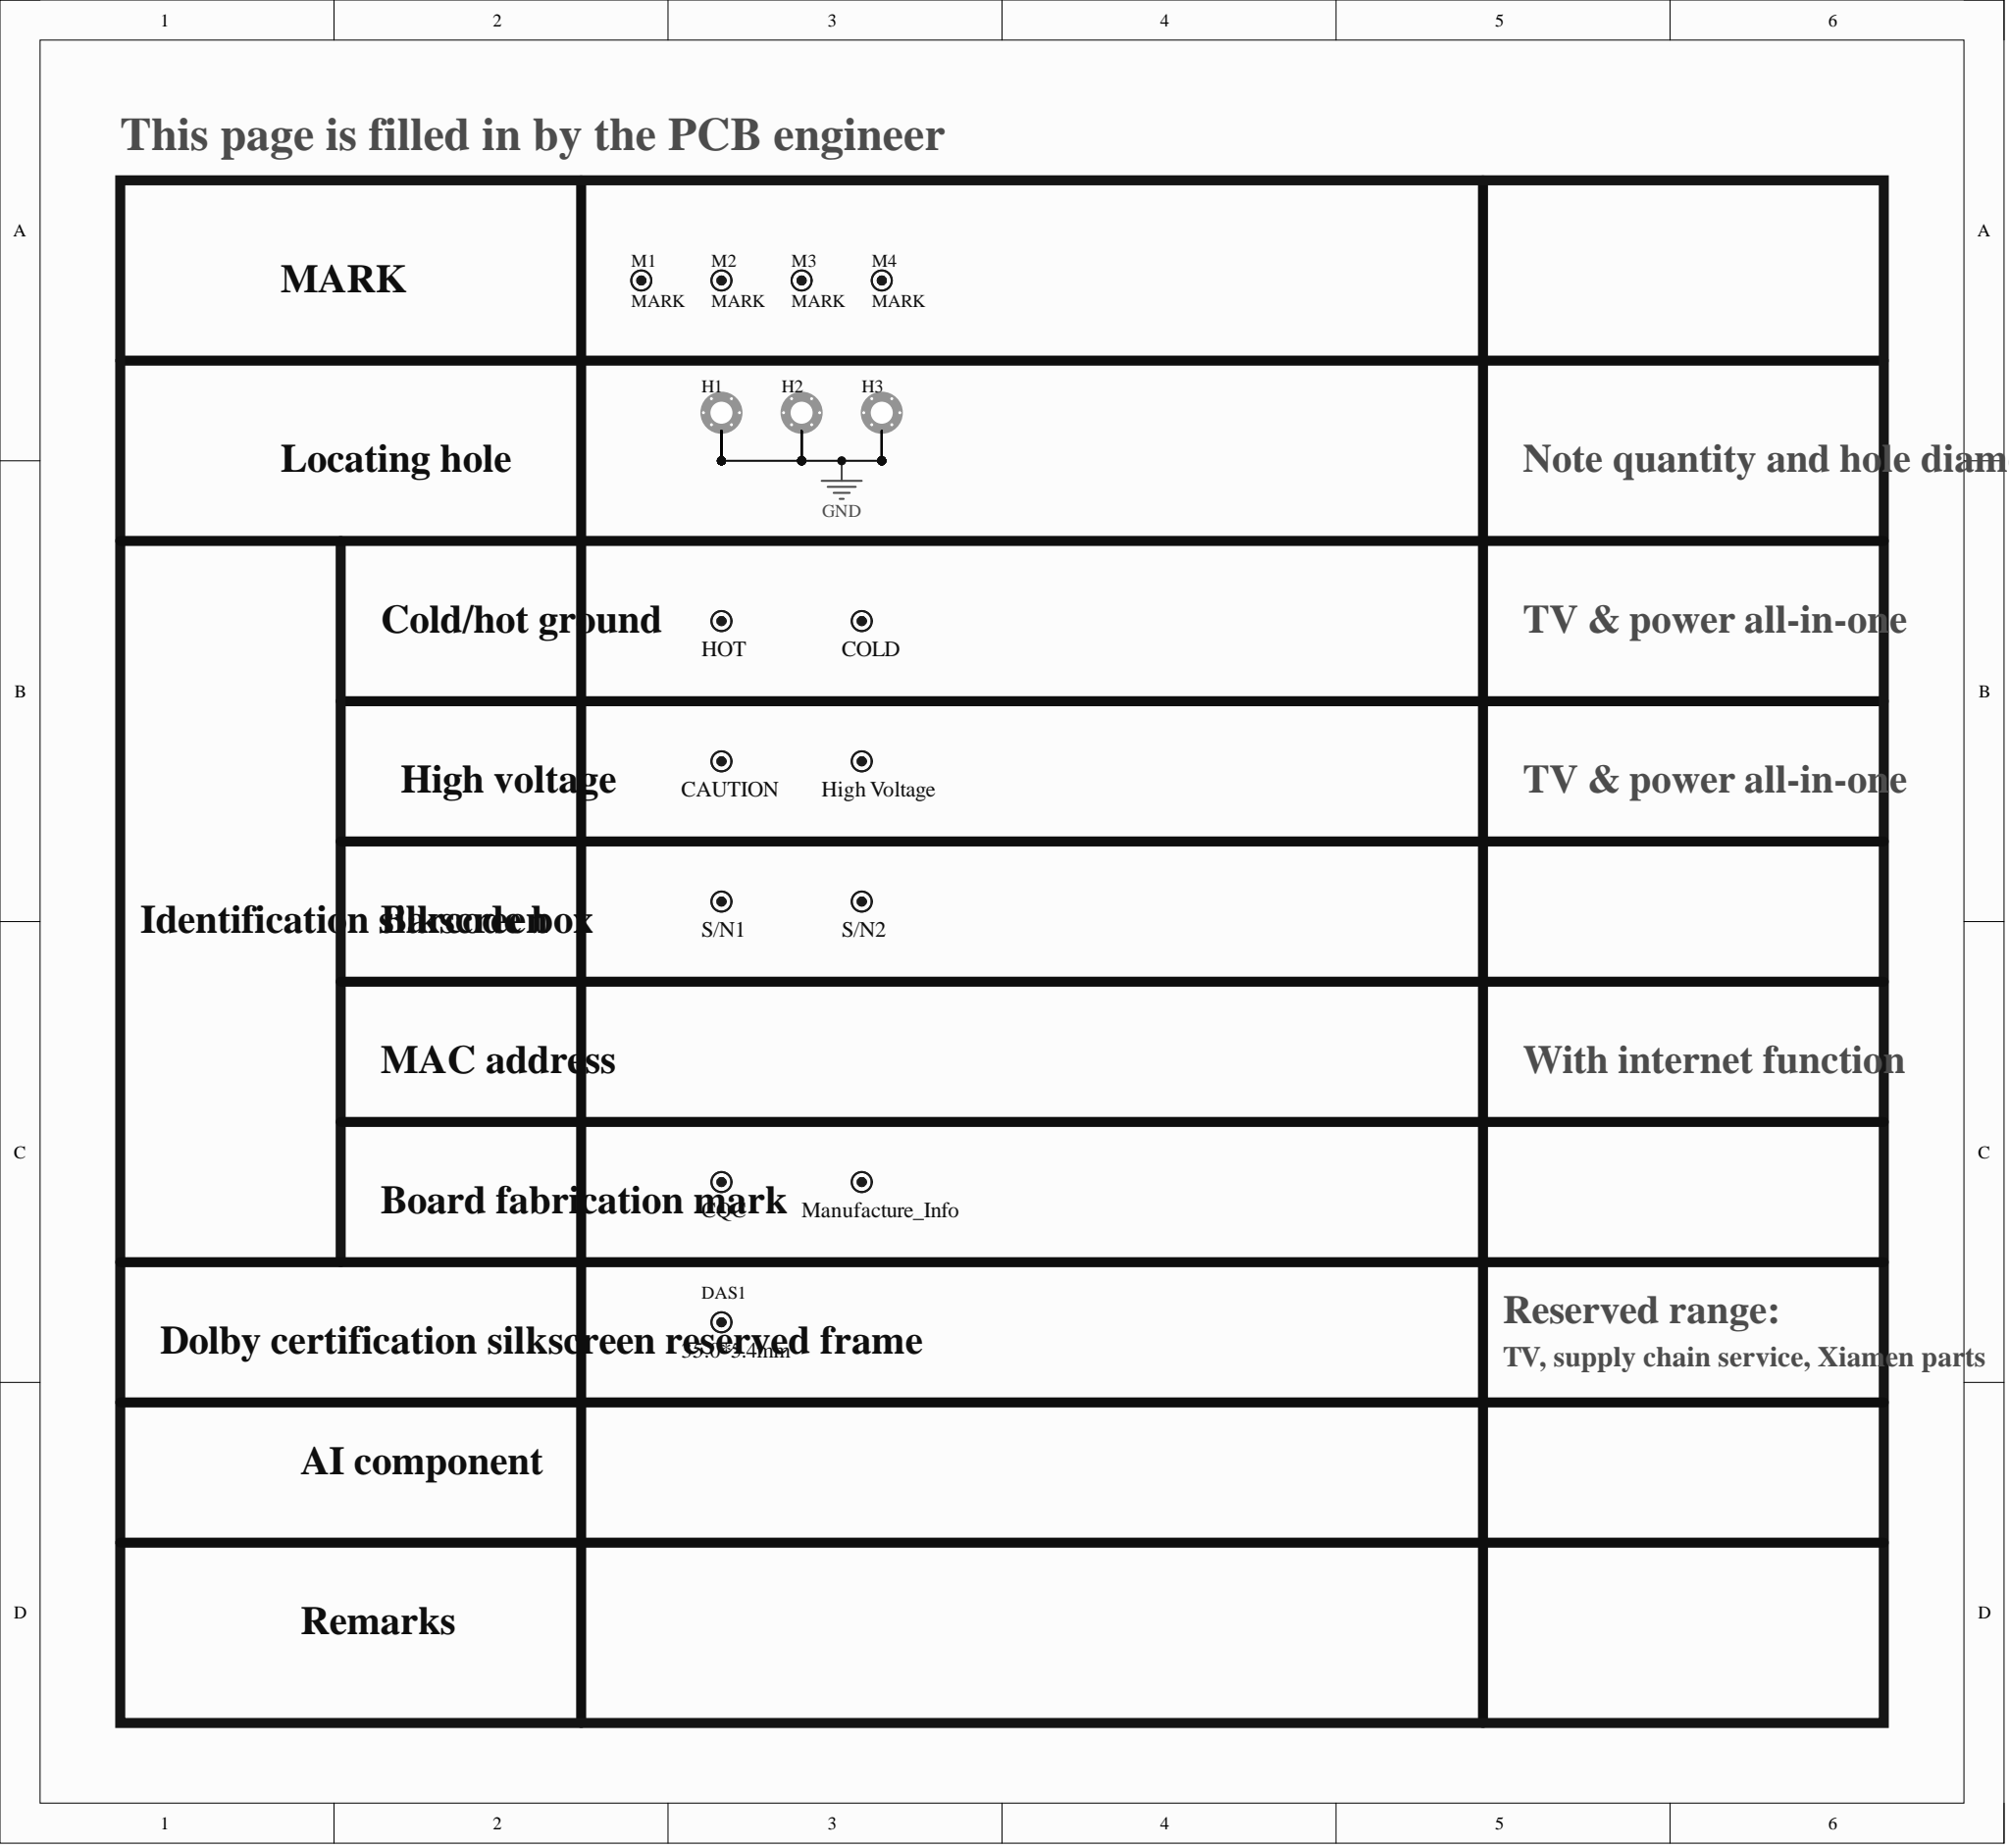Circuit board | Altium Designer | 527 parts | 243 nets | one sheet of the schematic
Parts on this sheet (reference | value | footprint):
CAUTION | CAUTION | CAUTION
COLD | COLD | COLD
CQC | CQC | CQC
DAS1 | 35.0*5.4mm | DOLBY_AS2
H1 | Location hole | ASSE4.0C-3
H2 | Location hole | ASSE4.0C-3
H3 | Location hole | ASSE4.0C-3
HOT | HOT | HOT
M1 | MARK | MARK
M2 | MARK | MARK
M3 | MARK | MARK
M4 | MARK | MARK
Manufacture_Info | Manufacture_Info | Manufacture_Info
S/N1 | Barcode | Barcode
S/N2 | Barcode | Barcode
Nets of these parts (net: part-pin ...):
GND: H1-1 H1-2 H1-3 H1-4 H1-5 H1-6 H2-1 H2-2 H2-3 H2-4 H2-5 H2-6 H3-1 H3-2 H3-3 H3-4 H3-5 H3-6